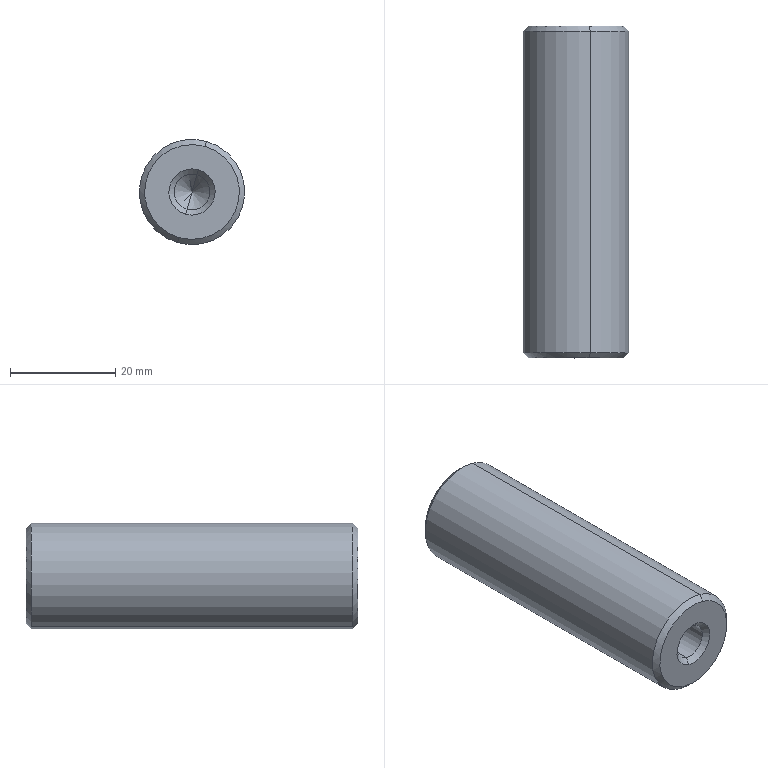Part | SolidWorks | features BaseBody 1 | 1 solid | 20 faces | box 20 x 63 x 20 mm | volume 18173 mm3 | cone 12 | cylinder 6 | plane 2 | commonest cylinder face diameters 6.8 x4 20 x2
STEP:
#1=CARTESIAN_POINT('',(-320.515,-34.5,751.3));
#2=VERTEX_POINT('',#1);
#3=CARTESIAN_POINT('',(-318.641,-34.5,757.836));
#4=VERTEX_POINT('',#3);
#5=CARTESIAN_POINT('',(-319.578,-34.5,754.568));
#6=DIRECTION('',(0.,1.,0.));
#7=DIRECTION('',(-0.2756,0.,-0.9613));
#8=AXIS2_PLACEMENT_3D('',#5,#6,#7);
#9=CIRCLE('',#8,3.4);
#10=EDGE_CURVE('',#2,#4,#9,.T.);
#11=ORIENTED_EDGE('',*,*,#10,.T.);
#12=CARTESIAN_POINT('',(-318.365,-35.5,758.798));
#13=VERTEX_POINT('',#12);
#14=CARTESIAN_POINT('',(-318.503,-35.,758.317));
#15=DIRECTION('',(0.1949,-0.7071,0.6797));
#16=VECTOR('',#15,1000.);
#17=LINE('',#14,#16);
#18=EDGE_CURVE('',#4,#13,#17,.T.);
#19=ORIENTED_EDGE('',*,*,#18,.T.);
#20=CARTESIAN_POINT('',(-320.791,-35.5,750.339));
#21=VERTEX_POINT('',#20);
#22=CARTESIAN_POINT('',(-319.578,-35.5,754.568));
#23=DIRECTION('',(0.,1.,0.));
#24=DIRECTION('',(-0.2756,0.,-0.9613));
#25=AXIS2_PLACEMENT_3D('',#22,#23,#24);
#26=CIRCLE('',#25,4.4);
#27=EDGE_CURVE('',#21,#13,#26,.T.);
#28=ORIENTED_EDGE('',*,*,#27,.F.);
#29=CARTESIAN_POINT('',(-320.653,-35.,750.819));
#30=DIRECTION('',(-0.1949,-0.7071,-0.6797));
#31=VECTOR('',#30,1000.);
#32=LINE('',#29,#31);
#33=EDGE_CURVE('',#2,#21,#32,.T.);
#34=ORIENTED_EDGE('',*,*,#33,.F.);
#35=EDGE_LOOP('',(#11,#19,#28,#34));
#36=FACE_OUTER_BOUND('',#35,.T.);
#37=CARTESIAN_POINT('',(-319.578,-35.,754.568));
#38=DIRECTION('',(0.,-1.,0.));
#39=DIRECTION('',(-0.2756,0.,-0.9613));
#40=AXIS2_PLACEMENT_3D('',#37,#38,#39);
#41=CONICAL_SURFACE('',#40,3.9,0.7854);
#42=ADVANCED_FACE('',(#36),#41,.F.);
#43=CARTESIAN_POINT('',(-318.641,-15.5,757.836));
#44=VERTEX_POINT('',#43);
#45=CARTESIAN_POINT('',(-320.515,-15.5,751.3));
#46=VERTEX_POINT('',#45);
#47=CARTESIAN_POINT('',(-319.578,-15.5,754.568));
#48=DIRECTION('',(0.,-1.,0.));
#49=DIRECTION('',(0.2756,0.,0.9613));
#50=AXIS2_PLACEMENT_3D('',#47,#48,#49);
#51=CIRCLE('',#50,3.4);
#52=EDGE_CURVE('',#44,#46,#51,.T.);
#53=ORIENTED_EDGE('',*,*,#52,.F.);
#54=CARTESIAN_POINT('',(-318.641,-15.5,757.836));
#55=DIRECTION('',(0.,-1.,0.));
#56=VECTOR('',#55,1000.);
#57=LINE('',#54,#56);
#58=EDGE_CURVE('',#44,#4,#57,.T.);
#59=ORIENTED_EDGE('',*,*,#58,.T.);
#60=ORIENTED_EDGE('',*,*,#10,.F.);
#61=CARTESIAN_POINT('',(-320.515,-15.5,751.3));
#62=DIRECTION('',(0.,-1.,0.));
#63=VECTOR('',#62,1000.);
#64=LINE('',#61,#63);
#65=EDGE_CURVE('',#46,#2,#64,.T.);
#66=ORIENTED_EDGE('',*,*,#65,.F.);
#67=EDGE_LOOP('',(#53,#59,#60,#66));
#68=FACE_OUTER_BOUND('',#67,.T.);
#69=CARTESIAN_POINT('',(-319.578,-15.5,754.568));
#70=DIRECTION('',(0.,-1.,0.));
#71=DIRECTION('',(-0.2756,0.,-0.9613));
#72=AXIS2_PLACEMENT_3D('',#69,#70,#71);
#73=CYLINDRICAL_SURFACE('',#72,3.4);
#74=ADVANCED_FACE('',(#68),#73,.F.);
#75=CARTESIAN_POINT('',(-319.578,-12.1,754.568));
#76=VERTEX_POINT('',#75);
#77=CARTESIAN_POINT('',(-320.056,-13.834,752.901));
#78=DIRECTION('',(-0.1949,-0.7071,-0.6797));
#79=VECTOR('',#78,1000.);
#80=LINE('',#77,#79);
#81=EDGE_CURVE('',#76,#46,#80,.T.);
#82=ORIENTED_EDGE('',*,*,#81,.F.);
#83=CARTESIAN_POINT('',(-319.1,-13.834,756.235));
#84=DIRECTION('',(0.1949,-0.7071,0.6797));
#85=VECTOR('',#84,1000.);
#86=LINE('',#83,#85);
#87=EDGE_CURVE('',#76,#44,#86,.T.);
#88=ORIENTED_EDGE('',*,*,#87,.T.);
#89=ORIENTED_EDGE('',*,*,#52,.T.);
#90=EDGE_LOOP('',(#82,#88,#89));
#91=FACE_OUTER_BOUND('',#90,.T.);
#92=CARTESIAN_POINT('',(-319.578,-13.834,754.568));
#93=DIRECTION('',(0.,-1.,0.));
#94=DIRECTION('',(-0.2756,0.,-0.9613));
#95=AXIS2_PLACEMENT_3D('',#92,#93,#94);
#96=CONICAL_SURFACE('',#95,1.734,0.7854);
#97=ADVANCED_FACE('',(#91),#96,.F.);
#98=CARTESIAN_POINT('',(-322.335,-34.5,744.956));
#99=VERTEX_POINT('',#98);
#100=CARTESIAN_POINT('',(-316.822,-34.5,764.181));
#101=VERTEX_POINT('',#100);
#102=CARTESIAN_POINT('',(-319.578,-34.5,754.568));
#103=DIRECTION('',(0.,-1.,0.));
#104=DIRECTION('',(-0.2756,0.,-0.9613));
#105=AXIS2_PLACEMENT_3D('',#102,#103,#104);
#106=CIRCLE('',#105,10.);
#107=EDGE_CURVE('',#99,#101,#106,.T.);
#108=ORIENTED_EDGE('',*,*,#107,.F.);
#109=CARTESIAN_POINT('',(-322.335,26.5,744.956));
#110=VERTEX_POINT('',#109);
#111=CARTESIAN_POINT('',(-322.335,-31.5,744.956));
#112=DIRECTION('',(0.,1.,0.));
#113=VECTOR('',#112,1000.);
#114=LINE('',#111,#113);
#115=EDGE_CURVE('',#99,#110,#114,.T.);
#116=ORIENTED_EDGE('',*,*,#115,.T.);
#117=CARTESIAN_POINT('',(-316.822,26.5,764.181));
#118=VERTEX_POINT('',#117);
#119=CARTESIAN_POINT('',(-319.578,26.5,754.568));
#120=DIRECTION('',(0.,1.,0.));
#121=DIRECTION('',(0.2756,0.,0.9613));
#122=AXIS2_PLACEMENT_3D('',#119,#120,#121);
#123=CIRCLE('',#122,10.);
#124=EDGE_CURVE('',#118,#110,#123,.T.);
#125=ORIENTED_EDGE('',*,*,#124,.F.);
#126=CARTESIAN_POINT('',(-316.822,-31.5,764.181));
#127=DIRECTION('',(0.,1.,0.));
#128=VECTOR('',#127,1000.);
#129=LINE('',#126,#128);
#130=EDGE_CURVE('',#101,#118,#129,.T.);
#131=ORIENTED_EDGE('',*,*,#130,.F.);
#132=EDGE_LOOP('',(#108,#116,#125,#131));
#133=FACE_OUTER_BOUND('',#132,.T.);
#134=CARTESIAN_POINT('',(-319.578,-31.5,754.568));
#135=DIRECTION('',(0.,1.,0.));
#136=DIRECTION('',(0.2756,0.,0.9613));
#137=AXIS2_PLACEMENT_3D('',#134,#135,#136);
#138=CYLINDRICAL_SURFACE('',#137,10.);
#139=ADVANCED_FACE('',(#133),#138,.T.);
#140=CARTESIAN_POINT('',(-322.059,-35.5,745.917));
#141=VERTEX_POINT('',#140);
#142=CARTESIAN_POINT('',(-317.097,-35.5,763.22));
#143=VERTEX_POINT('',#142);
#144=CARTESIAN_POINT('',(-319.578,-35.5,754.568));
#145=DIRECTION('',(0.,-1.,0.));
#146=DIRECTION('',(-0.2756,0.,-0.9613));
#147=AXIS2_PLACEMENT_3D('',#144,#145,#146);
#148=CIRCLE('',#147,9.);
#149=EDGE_CURVE('',#141,#143,#148,.T.);
#150=ORIENTED_EDGE('',*,*,#149,.F.);
#151=CARTESIAN_POINT('',(-322.197,-35.,745.436));
#152=DIRECTION('',(-0.1949,0.7071,-0.6797));
#153=VECTOR('',#152,1000.);
#154=LINE('',#151,#153);
#155=EDGE_CURVE('',#141,#99,#154,.T.);
#156=ORIENTED_EDGE('',*,*,#155,.T.);
#157=ORIENTED_EDGE('',*,*,#107,.T.);
#158=CARTESIAN_POINT('',(-316.96,-35.,763.7));
#159=DIRECTION('',(0.1949,0.7071,0.6797));
#160=VECTOR('',#159,1000.);
#161=LINE('',#158,#160);
#162=EDGE_CURVE('',#143,#101,#161,.T.);
#163=ORIENTED_EDGE('',*,*,#162,.F.);
#164=EDGE_LOOP('',(#150,#156,#157,#163));
#165=FACE_OUTER_BOUND('',#164,.T.);
#166=CARTESIAN_POINT('',(-319.578,-35.,754.568));
#167=DIRECTION('',(0.,1.,0.));
#168=DIRECTION('',(0.2756,0.,0.9613));
#169=AXIS2_PLACEMENT_3D('',#166,#167,#168);
#170=CONICAL_SURFACE('',#169,9.5,0.7854);
#171=ADVANCED_FACE('',(#165),#170,.T.);
#172=CARTESIAN_POINT('',(-317.097,27.5,763.22));
#173=VERTEX_POINT('',#172);
#174=CARTESIAN_POINT('',(-322.059,27.5,745.917));
#175=VERTEX_POINT('',#174);
#176=CARTESIAN_POINT('',(-319.578,27.5,754.568));
#177=DIRECTION('',(0.,1.,0.));
#178=DIRECTION('',(-0.2756,0.,-0.9613));
#179=AXIS2_PLACEMENT_3D('',#176,#177,#178);
#180=CIRCLE('',#179,9.);
#181=EDGE_CURVE('',#173,#175,#180,.T.);
#182=ORIENTED_EDGE('',*,*,#181,.F.);
#183=CARTESIAN_POINT('',(-316.96,27.,763.7));
#184=DIRECTION('',(0.1949,-0.7071,0.6797));
#185=VECTOR('',#184,1000.);
#186=LINE('',#183,#185);
#187=EDGE_CURVE('',#173,#118,#186,.T.);
#188=ORIENTED_EDGE('',*,*,#187,.T.);
#189=ORIENTED_EDGE('',*,*,#124,.T.);
#190=CARTESIAN_POINT('',(-322.197,27.,745.436));
#191=DIRECTION('',(-0.1949,-0.7071,-0.6797));
#192=VECTOR('',#191,1000.);
#193=LINE('',#190,#192);
#194=EDGE_CURVE('',#175,#110,#193,.T.);
#195=ORIENTED_EDGE('',*,*,#194,.F.);
#196=EDGE_LOOP('',(#182,#188,#189,#195));
#197=FACE_OUTER_BOUND('',#196,.T.);
#198=CARTESIAN_POINT('',(-319.578,27.,754.568));
#199=DIRECTION('',(0.,-1.,0.));
#200=DIRECTION('',(-0.2756,0.,-0.9613));
#201=AXIS2_PLACEMENT_3D('',#198,#199,#200);
#202=CONICAL_SURFACE('',#201,9.5,0.7854);
#203=ADVANCED_FACE('',(#197),#202,.T.);
#204=CARTESIAN_POINT('',(-320.515,7.5,751.3));
#205=VERTEX_POINT('',#204);
#206=CARTESIAN_POINT('',(-318.641,7.5,757.836));
#207=VERTEX_POINT('',#206);
#208=CARTESIAN_POINT('',(-319.578,7.5,754.568));
#209=DIRECTION('',(0.,1.,0.));
#210=DIRECTION('',(-0.2756,0.,-0.9613));
#211=AXIS2_PLACEMENT_3D('',#208,#209,#210);
#212=CIRCLE('',#211,3.4);
#213=EDGE_CURVE('',#205,#207,#212,.T.);
#214=ORIENTED_EDGE('',*,*,#213,.F.);
#215=CARTESIAN_POINT('',(-320.515,26.5,751.3));
#216=VERTEX_POINT('',#215);
#217=CARTESIAN_POINT('',(-320.515,7.5,751.3));
#218=DIRECTION('',(0.,1.,0.));
#219=VECTOR('',#218,1000.);
#220=LINE('',#217,#219);
#221=EDGE_CURVE('',#205,#216,#220,.T.);
#222=ORIENTED_EDGE('',*,*,#221,.T.);
#223=CARTESIAN_POINT('',(-318.641,26.5,757.836));
#224=VERTEX_POINT('',#223);
#225=CARTESIAN_POINT('',(-319.578,26.5,754.568));
#226=DIRECTION('',(0.,-1.,0.));
#227=DIRECTION('',(0.2756,0.,0.9613));
#228=AXIS2_PLACEMENT_3D('',#225,#226,#227);
#229=CIRCLE('',#228,3.4);
#230=EDGE_CURVE('',#224,#216,#229,.T.);
#231=ORIENTED_EDGE('',*,*,#230,.F.);
#232=CARTESIAN_POINT('',(-318.641,7.5,757.836));
#233=DIRECTION('',(0.,1.,0.));
#234=VECTOR('',#233,1000.);
#235=LINE('',#232,#234);
#236=EDGE_CURVE('',#207,#224,#235,.T.);
#237=ORIENTED_EDGE('',*,*,#236,.F.);
#238=EDGE_LOOP('',(#214,#222,#231,#237));
#239=FACE_OUTER_BOUND('',#238,.T.);
#240=CARTESIAN_POINT('',(-319.578,7.5,754.568));
#241=DIRECTION('',(0.,1.,0.));
#242=DIRECTION('',(0.2756,0.,0.9613));
#243=AXIS2_PLACEMENT_3D('',#240,#241,#242);
#244=CYLINDRICAL_SURFACE('',#243,3.4);
#245=ADVANCED_FACE('',(#239),#244,.F.);
#246=CARTESIAN_POINT('',(-319.578,4.1,754.568));
#247=VERTEX_POINT('',#246);
#248=CARTESIAN_POINT('',(-319.1,5.834,756.235));
#249=DIRECTION('',(0.1949,0.7071,0.6797));
#250=VECTOR('',#249,1000.);
#251=LINE('',#248,#250);
#252=EDGE_CURVE('',#247,#207,#251,.T.);
#253=ORIENTED_EDGE('',*,*,#252,.F.);
#254=CARTESIAN_POINT('',(-320.056,5.834,752.901));
#255=DIRECTION('',(-0.1949,0.7071,-0.6797));
#256=VECTOR('',#255,1000.);
#257=LINE('',#254,#256);
#258=EDGE_CURVE('',#247,#205,#257,.T.);
#259=ORIENTED_EDGE('',*,*,#258,.T.);
#260=ORIENTED_EDGE('',*,*,#213,.T.);
#261=EDGE_LOOP('',(#253,#259,#260));
#262=FACE_OUTER_BOUND('',#261,.T.);
#263=CARTESIAN_POINT('',(-319.578,5.834,754.568));
#264=DIRECTION('',(0.,1.,0.));
#265=DIRECTION('',(0.2756,0.,0.9613));
#266=AXIS2_PLACEMENT_3D('',#263,#264,#265);
#267=CONICAL_SURFACE('',#266,1.734,0.7854);
#268=ADVANCED_FACE('',(#262),#267,.F.);
#269=ORIENTED_EDGE('',*,*,#230,.T.);
#270=CARTESIAN_POINT('',(-320.791,27.5,750.339));
#271=VERTEX_POINT('',#270);
#272=CARTESIAN_POINT('',(-320.653,27.,750.819));
#273=DIRECTION('',(-0.1949,0.7071,-0.6797));
#274=VECTOR('',#273,1000.);
#275=LINE('',#272,#274);
#276=EDGE_CURVE('',#216,#271,#275,.T.);
#277=ORIENTED_EDGE('',*,*,#276,.T.);
#278=CARTESIAN_POINT('',(-318.365,27.5,758.798));
#279=VERTEX_POINT('',#278);
#280=CARTESIAN_POINT('',(-319.578,27.5,754.568));
#281=DIRECTION('',(0.,-1.,0.));
#282=DIRECTION('',(0.2756,0.,0.9613));
#283=AXIS2_PLACEMENT_3D('',#280,#281,#282);
#284=CIRCLE('',#283,4.4);
#285=EDGE_CURVE('',#279,#271,#284,.T.);
#286=ORIENTED_EDGE('',*,*,#285,.F.);
#287=CARTESIAN_POINT('',(-318.503,27.,758.317));
#288=DIRECTION('',(0.1949,0.7071,0.6797));
#289=VECTOR('',#288,1000.);
#290=LINE('',#287,#289);
#291=EDGE_CURVE('',#224,#279,#290,.T.);
#292=ORIENTED_EDGE('',*,*,#291,.F.);
#293=EDGE_LOOP('',(#269,#277,#286,#292));
#294=FACE_OUTER_BOUND('',#293,.T.);
#295=CARTESIAN_POINT('',(-319.578,27.,754.568));
#296=DIRECTION('',(0.,1.,0.));
#297=DIRECTION('',(0.2756,0.,0.9613));
#298=AXIS2_PLACEMENT_3D('',#295,#296,#297);
#299=CONICAL_SURFACE('',#298,3.9,0.7854);
#300=ADVANCED_FACE('',(#294),#299,.F.);
#301=ORIENTED_EDGE('',*,*,#276,.F.);
#302=CARTESIAN_POINT('',(-319.578,26.5,754.568));
#303=DIRECTION('',(0.,-1.,0.));
#304=DIRECTION('',(0.2756,0.,0.9613));
#305=AXIS2_PLACEMENT_3D('',#302,#303,#304);
#306=CIRCLE('',#305,3.4);
#307=EDGE_CURVE('',#216,#224,#306,.T.);
#308=ORIENTED_EDGE('',*,*,#307,.T.);
#309=ORIENTED_EDGE('',*,*,#291,.T.);
#310=CARTESIAN_POINT('',(-319.578,27.5,754.568));
#311=DIRECTION('',(0.,-1.,0.));
#312=DIRECTION('',(0.2756,0.,0.9613));
#313=AXIS2_PLACEMENT_3D('',#310,#311,#312);
#314=CIRCLE('',#313,4.4);
#315=EDGE_CURVE('',#271,#279,#314,.T.);
#316=ORIENTED_EDGE('',*,*,#315,.F.);
#317=EDGE_LOOP('',(#301,#308,#309,#316));
#318=FACE_OUTER_BOUND('',#317,.T.);
#319=CARTESIAN_POINT('',(-319.578,27.,754.568));
#320=DIRECTION('',(0.,1.,0.));
#321=DIRECTION('',(0.2756,0.,0.9613));
#322=AXIS2_PLACEMENT_3D('',#319,#320,#321);
#323=CONICAL_SURFACE('',#322,3.9,0.7854);
#324=ADVANCED_FACE('',(#318),#323,.F.);
#325=ORIENTED_EDGE('',*,*,#258,.F.);
#326=ORIENTED_EDGE('',*,*,#252,.T.);
#327=CARTESIAN_POINT('',(-319.578,7.5,754.568));
#328=DIRECTION('',(0.,1.,0.));
#329=DIRECTION('',(-0.2756,0.,-0.9613));
#330=AXIS2_PLACEMENT_3D('',#327,#328,#329);
#331=CIRCLE('',#330,3.4);
#332=EDGE_CURVE('',#207,#205,#331,.T.);
#333=ORIENTED_EDGE('',*,*,#332,.T.);
#334=EDGE_LOOP('',(#325,#326,#333));
#335=FACE_OUTER_BOUND('',#334,.T.);
#336=CARTESIAN_POINT('',(-319.578,5.834,754.568));
#337=DIRECTION('',(0.,1.,0.));
#338=DIRECTION('',(0.2756,0.,0.9613));
#339=AXIS2_PLACEMENT_3D('',#336,#337,#338);
#340=CONICAL_SURFACE('',#339,1.734,0.7854);
#341=ADVANCED_FACE('',(#335),#340,.F.);
#342=ORIENTED_EDGE('',*,*,#221,.F.);
#343=ORIENTED_EDGE('',*,*,#332,.F.);
#344=ORIENTED_EDGE('',*,*,#236,.T.);
#345=ORIENTED_EDGE('',*,*,#307,.F.);
#346=EDGE_LOOP('',(#342,#343,#344,#345));
#347=FACE_OUTER_BOUND('',#346,.T.);
#348=CARTESIAN_POINT('',(-319.578,7.5,754.568));
#349=DIRECTION('',(0.,1.,0.));
#350=DIRECTION('',(0.2756,0.,0.9613));
#351=AXIS2_PLACEMENT_3D('',#348,#349,#350);
#352=CYLINDRICAL_SURFACE('',#351,3.4);
#353=ADVANCED_FACE('',(#347),#352,.F.);
#354=ORIENTED_EDGE('',*,*,#285,.T.);
#355=ORIENTED_EDGE('',*,*,#315,.T.);
#356=EDGE_LOOP('',(#354,#355));
#357=FACE_BOUND('',#356,.T.);
#358=CARTESIAN_POINT('',(-319.578,27.5,754.568));
#359=DIRECTION('',(0.,1.,0.));
#360=DIRECTION('',(-0.2756,0.,-0.9613));
#361=AXIS2_PLACEMENT_3D('',#358,#359,#360);
#362=CIRCLE('',#361,9.);
#363=EDGE_CURVE('',#175,#173,#362,.T.);
#364=ORIENTED_EDGE('',*,*,#363,.T.);
#365=ORIENTED_EDGE('',*,*,#181,.T.);
#366=EDGE_LOOP('',(#364,#365));
#367=FACE_OUTER_BOUND('',#366,.T.);
#368=CARTESIAN_POINT('',(-319.578,27.5,754.568));
#369=DIRECTION('',(0.,-1.,0.));
#370=DIRECTION('',(0.,0.,-1.));
#371=AXIS2_PLACEMENT_3D('',#368,#369,#370);
#372=PLANE('',#371);
#373=ADVANCED_FACE('',(#357,#367),#372,.F.);
#374=ORIENTED_EDGE('',*,*,#187,.F.);
#375=ORIENTED_EDGE('',*,*,#363,.F.);
#376=ORIENTED_EDGE('',*,*,#194,.T.);
#377=CARTESIAN_POINT('',(-319.578,26.5,754.568));
#378=DIRECTION('',(0.,1.,0.));
#379=DIRECTION('',(0.2756,0.,0.9613));
#380=AXIS2_PLACEMENT_3D('',#377,#378,#379);
#381=CIRCLE('',#380,10.);
#382=EDGE_CURVE('',#110,#118,#381,.T.);
#383=ORIENTED_EDGE('',*,*,#382,.T.);
#384=EDGE_LOOP('',(#374,#375,#376,#383));
#385=FACE_OUTER_BOUND('',#384,.T.);
#386=CARTESIAN_POINT('',(-319.578,27.,754.568));
#387=DIRECTION('',(0.,-1.,0.));
#388=DIRECTION('',(-0.2756,0.,-0.9613));
#389=AXIS2_PLACEMENT_3D('',#386,#387,#388);
#390=CONICAL_SURFACE('',#389,9.5,0.7854);
#391=ADVANCED_FACE('',(#385),#390,.T.);
#392=ORIENTED_EDGE('',*,*,#27,.T.);
#393=CARTESIAN_POINT('',(-319.578,-35.5,754.568));
#394=DIRECTION('',(0.,1.,0.));
#395=DIRECTION('',(-0.2756,0.,-0.9613));
#396=AXIS2_PLACEMENT_3D('',#393,#394,#395);
#397=CIRCLE('',#396,4.4);
#398=EDGE_CURVE('',#13,#21,#397,.T.);
#399=ORIENTED_EDGE('',*,*,#398,.T.);
#400=EDGE_LOOP('',(#392,#399));
#401=FACE_BOUND('',#400,.T.);
#402=CARTESIAN_POINT('',(-319.578,-35.5,754.568));
#403=DIRECTION('',(0.,-1.,0.));
#404=DIRECTION('',(-0.2756,0.,-0.9613));
#405=AXIS2_PLACEMENT_3D('',#402,#403,#404);
#406=CIRCLE('',#405,9.);
#407=EDGE_CURVE('',#143,#141,#406,.T.);
#408=ORIENTED_EDGE('',*,*,#407,.T.);
#409=ORIENTED_EDGE('',*,*,#149,.T.);
#410=EDGE_LOOP('',(#408,#409));
#411=FACE_OUTER_BOUND('',#410,.T.);
#412=CARTESIAN_POINT('',(-319.578,-35.5,754.568));
#413=DIRECTION('',(0.,-1.,0.));
#414=DIRECTION('',(0.,0.,-1.));
#415=AXIS2_PLACEMENT_3D('',#412,#413,#414);
#416=PLANE('',#415);
#417=ADVANCED_FACE('',(#401,#411),#416,.T.);
#418=ORIENTED_EDGE('',*,*,#155,.F.);
#419=ORIENTED_EDGE('',*,*,#407,.F.);
#420=ORIENTED_EDGE('',*,*,#162,.T.);
#421=CARTESIAN_POINT('',(-319.578,-34.5,754.568));
#422=DIRECTION('',(0.,-1.,0.));
#423=DIRECTION('',(-0.2756,0.,-0.9613));
#424=AXIS2_PLACEMENT_3D('',#421,#422,#423);
#425=CIRCLE('',#424,10.);
#426=EDGE_CURVE('',#101,#99,#425,.T.);
#427=ORIENTED_EDGE('',*,*,#426,.T.);
#428=EDGE_LOOP('',(#418,#419,#420,#427));
#429=FACE_OUTER_BOUND('',#428,.T.);
#430=CARTESIAN_POINT('',(-319.578,-35.,754.568));
#431=DIRECTION('',(0.,1.,0.));
#432=DIRECTION('',(0.2756,0.,0.9613));
#433=AXIS2_PLACEMENT_3D('',#430,#431,#432);
#434=CONICAL_SURFACE('',#433,9.5,0.7854);
#435=ADVANCED_FACE('',(#429),#434,.T.);
#436=ORIENTED_EDGE('',*,*,#115,.F.);
#437=ORIENTED_EDGE('',*,*,#426,.F.);
#438=ORIENTED_EDGE('',*,*,#130,.T.);
#439=ORIENTED_EDGE('',*,*,#382,.F.);
#440=EDGE_LOOP('',(#436,#437,#438,#439));
#441=FACE_OUTER_BOUND('',#440,.T.);
#442=CARTESIAN_POINT('',(-319.578,-31.5,754.568));
#443=DIRECTION('',(0.,1.,0.));
#444=DIRECTION('',(0.2756,0.,0.9613));
#445=AXIS2_PLACEMENT_3D('',#442,#443,#444);
#446=CYLINDRICAL_SURFACE('',#445,10.);
#447=ADVANCED_FACE('',(#441),#446,.T.);
#448=ORIENTED_EDGE('',*,*,#87,.F.);
#449=ORIENTED_EDGE('',*,*,#81,.T.);
#450=CARTESIAN_POINT('',(-319.578,-15.5,754.568));
#451=DIRECTION('',(0.,-1.,0.));
#452=DIRECTION('',(0.2756,0.,0.9613));
#453=AXIS2_PLACEMENT_3D('',#450,#451,#452);
#454=CIRCLE('',#453,3.4);
#455=EDGE_CURVE('',#46,#44,#454,.T.);
#456=ORIENTED_EDGE('',*,*,#455,.T.);
#457=EDGE_LOOP('',(#448,#449,#456));
#458=FACE_OUTER_BOUND('',#457,.T.);
#459=CARTESIAN_POINT('',(-319.578,-13.834,754.568));
#460=DIRECTION('',(0.,-1.,0.));
#461=DIRECTION('',(-0.2756,0.,-0.9613));
#462=AXIS2_PLACEMENT_3D('',#459,#460,#461);
#463=CONICAL_SURFACE('',#462,1.734,0.7854);
#464=ADVANCED_FACE('',(#458),#463,.F.);
#465=ORIENTED_EDGE('',*,*,#58,.F.);
#466=ORIENTED_EDGE('',*,*,#455,.F.);
#467=ORIENTED_EDGE('',*,*,#65,.T.);
#468=CARTESIAN_POINT('',(-319.578,-34.5,754.568));
#469=DIRECTION('',(0.,1.,0.));
#470=DIRECTION('',(-0.2756,0.,-0.9613));
#471=AXIS2_PLACEMENT_3D('',#468,#469,#470);
#472=CIRCLE('',#471,3.4);
#473=EDGE_CURVE('',#4,#2,#472,.T.);
#474=ORIENTED_EDGE('',*,*,#473,.F.);
#475=EDGE_LOOP('',(#465,#466,#467,#474));
#476=FACE_OUTER_BOUND('',#475,.T.);
#477=CARTESIAN_POINT('',(-319.578,-15.5,754.568));
#478=DIRECTION('',(0.,-1.,0.));
#479=DIRECTION('',(-0.2756,0.,-0.9613));
#480=AXIS2_PLACEMENT_3D('',#477,#478,#479);
#481=CYLINDRICAL_SURFACE('',#480,3.4);
#482=ADVANCED_FACE('',(#476),#481,.F.);
#483=ORIENTED_EDGE('',*,*,#18,.F.);
#484=ORIENTED_EDGE('',*,*,#473,.T.);
#485=ORIENTED_EDGE('',*,*,#33,.T.);
#486=ORIENTED_EDGE('',*,*,#398,.F.);
#487=EDGE_LOOP('',(#483,#484,#485,#486));
#488=FACE_OUTER_BOUND('',#487,.T.);
#489=CARTESIAN_POINT('',(-319.578,-35.,754.568));
#490=DIRECTION('',(0.,-1.,0.));
#491=DIRECTION('',(-0.2756,0.,-0.9613));
#492=AXIS2_PLACEMENT_3D('',#489,#490,#491);
#493=CONICAL_SURFACE('',#492,3.9,0.7854);
#494=ADVANCED_FACE('',(#488),#493,.F.);
#495=CLOSED_SHELL('',(#42,#74,#97,#139,#171,#203,#245,#268,#300,#324,#341,#353,#373,#391,#417,#435,#447,#464,#482,#494));
#496=MANIFOLD_SOLID_BREP('',#495);
#497=CARTESIAN_POINT('',(0.,0.,0.));
#498=DIRECTION('',(0.,0.,1.));
#499=DIRECTION('',(1.,0.,0.));
#500=AXIS2_PLACEMENT_3D('',#497,#498,#499);
#501=(LENGTH_UNIT()NAMED_UNIT(*)SI_UNIT(.MILLI.,.METRE.));
#502=UNCERTAINTY_MEASURE_WITH_UNIT(LENGTH_MEASURE(0.00001),#501,'','');
#503=(NAMED_UNIT(*)PLANE_ANGLE_UNIT()SI_UNIT($,.RADIAN.));
#504=(NAMED_UNIT(*)SI_UNIT($,.STERADIAN.)SOLID_ANGLE_UNIT());
#505=(GEOMETRIC_REPRESENTATION_CONTEXT(3)GLOBAL_UNCERTAINTY_ASSIGNED_CONTEXT((#502))GLOBAL_UNIT_ASSIGNED_CONTEXT((#501,#503,#504))REPRESENTATION_CONTEXT('',''));
#506=ADVANCED_BREP_SHAPE_REPRESENTATION('',(#496,#500),#505);